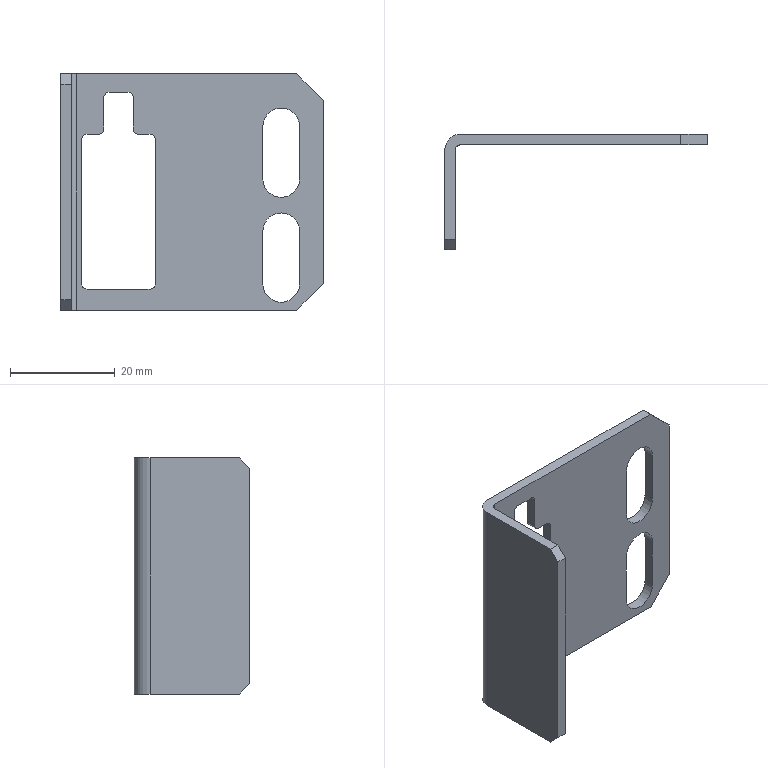Part | STEP file | 1358-7.stp.STEP | 1 solid | 40 faces | box 50 x 22 x 45 mm | volume 4817 mm3 | plane 24 | cylinder 16 | commonest cylinder face diameters 2 x9 7 x6 6 x1
STEP:
#1=CARTESIAN_POINT('',(0.,22.,20.));
#2=VERTEX_POINT('',#1);
#3=CARTESIAN_POINT('',(0.,5.,20.));
#4=VERTEX_POINT('',#3);
#5=CARTESIAN_POINT('',(0.,22.,20.));
#6=DIRECTION('',(0.,-1.,0.));
#7=VECTOR('',#6,1000.);
#8=LINE('',#5,#7);
#9=EDGE_CURVE('',#2,#4,#8,.T.);
#10=ORIENTED_EDGE('',*,*,#9,.T.);
#11=CARTESIAN_POINT('',(2.,5.,20.));
#12=VERTEX_POINT('',#11);
#13=CARTESIAN_POINT('',(2.,5.,20.));
#14=DIRECTION('',(-1.,0.,0.));
#15=VECTOR('',#14,1000.);
#16=LINE('',#13,#15);
#17=EDGE_CURVE('',#12,#4,#16,.T.);
#18=ORIENTED_EDGE('',*,*,#17,.F.);
#19=CARTESIAN_POINT('',(2.,22.,20.));
#20=VERTEX_POINT('',#19);
#21=CARTESIAN_POINT('',(2.,22.,20.));
#22=DIRECTION('',(0.,-1.,0.));
#23=VECTOR('',#22,1000.);
#24=LINE('',#21,#23);
#25=EDGE_CURVE('',#20,#12,#24,.T.);
#26=ORIENTED_EDGE('',*,*,#25,.F.);
#27=CARTESIAN_POINT('',(3.,23.,20.));
#28=VERTEX_POINT('',#27);
#29=CARTESIAN_POINT('',(3.,22.,20.));
#30=DIRECTION('',(0.,0.,-1.));
#31=DIRECTION('',(-1.,0.,0.));
#32=AXIS2_PLACEMENT_3D('',#29,#30,#31);
#33=CIRCLE('',#32,1.);
#34=EDGE_CURVE('',#20,#28,#33,.T.);
#35=ORIENTED_EDGE('',*,*,#34,.T.);
#36=CARTESIAN_POINT('',(45.,23.,20.));
#37=VERTEX_POINT('',#36);
#38=CARTESIAN_POINT('',(3.,23.,20.));
#39=DIRECTION('',(1.,0.,0.));
#40=VECTOR('',#39,1000.);
#41=LINE('',#38,#40);
#42=EDGE_CURVE('',#28,#37,#41,.T.);
#43=ORIENTED_EDGE('',*,*,#42,.T.);
#44=CARTESIAN_POINT('',(45.,25.,20.));
#45=VERTEX_POINT('',#44);
#46=CARTESIAN_POINT('',(45.,25.,20.));
#47=DIRECTION('',(0.,-1.,0.));
#48=VECTOR('',#47,1000.);
#49=LINE('',#46,#48);
#50=EDGE_CURVE('',#45,#37,#49,.T.);
#51=ORIENTED_EDGE('',*,*,#50,.F.);
#52=CARTESIAN_POINT('',(3.,25.,20.));
#53=VERTEX_POINT('',#52);
#54=CARTESIAN_POINT('',(3.,25.,20.));
#55=DIRECTION('',(1.,0.,0.));
#56=VECTOR('',#55,1000.);
#57=LINE('',#54,#56);
#58=EDGE_CURVE('',#53,#45,#57,.T.);
#59=ORIENTED_EDGE('',*,*,#58,.F.);
#60=CARTESIAN_POINT('',(3.,22.,20.));
#61=DIRECTION('',(0.,0.,1.));
#62=DIRECTION('',(0.,1.,0.));
#63=AXIS2_PLACEMENT_3D('',#60,#61,#62);
#64=CIRCLE('',#63,3.);
#65=EDGE_CURVE('',#53,#2,#64,.T.);
#66=ORIENTED_EDGE('',*,*,#65,.T.);
#67=EDGE_LOOP('',(#10,#18,#26,#35,#43,#51,#59,#66));
#68=FACE_OUTER_BOUND('',#67,.T.);
#69=CARTESIAN_POINT('',(0.,0.,20.));
#70=DIRECTION('',(0.,0.,1.));
#71=DIRECTION('',(1.,0.,0.));
#72=AXIS2_PLACEMENT_3D('',#69,#70,#71);
#73=PLANE('',#72);
#74=ADVANCED_FACE('',(#68),#73,.T.);
#75=CARTESIAN_POINT('',(3.,25.,-25.));
#76=VERTEX_POINT('',#75);
#77=CARTESIAN_POINT('',(3.,25.,-25.));
#78=DIRECTION('',(0.,0.,1.));
#79=VECTOR('',#78,1000.);
#80=LINE('',#77,#79);
#81=EDGE_CURVE('',#76,#53,#80,.T.);
#82=ORIENTED_EDGE('',*,*,#81,.F.);
#83=CARTESIAN_POINT('',(0.,22.,-25.));
#84=VERTEX_POINT('',#83);
#85=CARTESIAN_POINT('',(3.,22.,-25.));
#86=DIRECTION('',(0.,0.,-1.));
#87=DIRECTION('',(-1.,0.,0.));
#88=AXIS2_PLACEMENT_3D('',#85,#86,#87);
#89=CIRCLE('',#88,3.);
#90=EDGE_CURVE('',#84,#76,#89,.T.);
#91=ORIENTED_EDGE('',*,*,#90,.F.);
#92=CARTESIAN_POINT('',(0.,22.,-25.));
#93=DIRECTION('',(0.,0.,1.));
#94=VECTOR('',#93,1000.);
#95=LINE('',#92,#94);
#96=EDGE_CURVE('',#84,#2,#95,.T.);
#97=ORIENTED_EDGE('',*,*,#96,.T.);
#98=ORIENTED_EDGE('',*,*,#65,.F.);
#99=EDGE_LOOP('',(#82,#91,#97,#98));
#100=FACE_OUTER_BOUND('',#99,.T.);
#101=CARTESIAN_POINT('',(3.,22.,-83.662));
#102=DIRECTION('',(0.,0.,1.));
#103=DIRECTION('',(0.,1.,0.));
#104=AXIS2_PLACEMENT_3D('',#101,#102,#103);
#105=CYLINDRICAL_SURFACE('',#104,3.);
#106=ADVANCED_FACE('',(#100),#105,.T.);
#107=CARTESIAN_POINT('',(0.,5.,-25.));
#108=VERTEX_POINT('',#107);
#109=CARTESIAN_POINT('',(0.,5.,-25.));
#110=DIRECTION('',(0.,1.,0.));
#111=VECTOR('',#110,1000.);
#112=LINE('',#109,#111);
#113=EDGE_CURVE('',#108,#84,#112,.T.);
#114=ORIENTED_EDGE('',*,*,#113,.F.);
#115=CARTESIAN_POINT('',(0.,3.,-23.));
#116=VERTEX_POINT('',#115);
#117=CARTESIAN_POINT('',(0.,5.,-25.));
#118=DIRECTION('',(0.,-0.7071,0.7071));
#119=VECTOR('',#118,1000.);
#120=LINE('',#117,#119);
#121=EDGE_CURVE('',#108,#116,#120,.T.);
#122=ORIENTED_EDGE('',*,*,#121,.T.);
#123=CARTESIAN_POINT('',(0.,3.,18.));
#124=VERTEX_POINT('',#123);
#125=CARTESIAN_POINT('',(0.,3.,18.));
#126=DIRECTION('',(0.,0.,-1.));
#127=VECTOR('',#126,1000.);
#128=LINE('',#125,#127);
#129=EDGE_CURVE('',#124,#116,#128,.T.);
#130=ORIENTED_EDGE('',*,*,#129,.F.);
#131=CARTESIAN_POINT('',(0.,3.,18.));
#132=DIRECTION('',(0.,0.7071,0.7071));
#133=VECTOR('',#132,1000.);
#134=LINE('',#131,#133);
#135=EDGE_CURVE('',#124,#4,#134,.T.);
#136=ORIENTED_EDGE('',*,*,#135,.T.);
#137=ORIENTED_EDGE('',*,*,#9,.F.);
#138=ORIENTED_EDGE('',*,*,#96,.F.);
#139=EDGE_LOOP('',(#114,#122,#130,#136,#137,#138));
#140=FACE_OUTER_BOUND('',#139,.T.);
#141=CARTESIAN_POINT('',(0.,25.,-20.));
#142=DIRECTION('',(-1.,0.,0.));
#143=DIRECTION('',(0.,0.,1.));
#144=AXIS2_PLACEMENT_3D('',#141,#142,#143);
#145=PLANE('',#144);
#146=ADVANCED_FACE('',(#140),#145,.T.);
#147=CARTESIAN_POINT('',(2.,3.,18.));
#148=VERTEX_POINT('',#147);
#149=CARTESIAN_POINT('',(2.,3.,18.));
#150=DIRECTION('',(-1.,0.,0.));
#151=VECTOR('',#150,1000.);
#152=LINE('',#149,#151);
#153=EDGE_CURVE('',#148,#124,#152,.T.);
#154=ORIENTED_EDGE('',*,*,#153,.F.);
#155=CARTESIAN_POINT('',(2.,5.,20.));
#156=DIRECTION('',(0.,-0.7071,-0.7071));
#157=VECTOR('',#156,1000.);
#158=LINE('',#155,#157);
#159=EDGE_CURVE('',#12,#148,#158,.T.);
#160=ORIENTED_EDGE('',*,*,#159,.F.);
#161=ORIENTED_EDGE('',*,*,#17,.T.);
#162=ORIENTED_EDGE('',*,*,#135,.F.);
#163=EDGE_LOOP('',(#154,#160,#161,#162));
#164=FACE_OUTER_BOUND('',#163,.T.);
#165=CARTESIAN_POINT('',(1.,4.,19.));
#166=DIRECTION('',(0.,-0.7071,0.7071));
#167=DIRECTION('',(-1.,0.,0.));
#168=AXIS2_PLACEMENT_3D('',#165,#166,#167);
#169=PLANE('',#168);
#170=ADVANCED_FACE('',(#164),#169,.T.);
#171=ORIENTED_EDGE('',*,*,#25,.T.);
#172=ORIENTED_EDGE('',*,*,#159,.T.);
#173=CARTESIAN_POINT('',(2.,3.,-23.));
#174=VERTEX_POINT('',#173);
#175=CARTESIAN_POINT('',(2.,3.,-23.));
#176=DIRECTION('',(0.,0.,1.));
#177=VECTOR('',#176,1000.);
#178=LINE('',#175,#177);
#179=EDGE_CURVE('',#174,#148,#178,.T.);
#180=ORIENTED_EDGE('',*,*,#179,.F.);
#181=CARTESIAN_POINT('',(2.,5.,-25.));
#182=VERTEX_POINT('',#181);
#183=CARTESIAN_POINT('',(2.,3.,-23.));
#184=DIRECTION('',(0.,0.7071,-0.7071));
#185=VECTOR('',#184,1000.);
#186=LINE('',#183,#185);
#187=EDGE_CURVE('',#174,#182,#186,.T.);
#188=ORIENTED_EDGE('',*,*,#187,.T.);
#189=CARTESIAN_POINT('',(2.,22.,-25.));
#190=VERTEX_POINT('',#189);
#191=CARTESIAN_POINT('',(2.,22.,-25.));
#192=DIRECTION('',(0.,-1.,0.));
#193=VECTOR('',#192,1000.);
#194=LINE('',#191,#193);
#195=EDGE_CURVE('',#190,#182,#194,.T.);
#196=ORIENTED_EDGE('',*,*,#195,.F.);
#197=CARTESIAN_POINT('',(2.,22.,-25.));
#198=DIRECTION('',(0.,0.,1.));
#199=VECTOR('',#198,1000.);
#200=LINE('',#197,#199);
#201=EDGE_CURVE('',#190,#20,#200,.T.);
#202=ORIENTED_EDGE('',*,*,#201,.T.);
#203=EDGE_LOOP('',(#171,#172,#180,#188,#196,#202));
#204=FACE_OUTER_BOUND('',#203,.T.);
#205=CARTESIAN_POINT('',(2.,23.,-25.));
#206=DIRECTION('',(1.,0.,0.));
#207=DIRECTION('',(0.,1.,0.));
#208=AXIS2_PLACEMENT_3D('',#205,#206,#207);
#209=PLANE('',#208);
#210=ADVANCED_FACE('',(#204),#209,.T.);
#211=ORIENTED_EDGE('',*,*,#34,.F.);
#212=ORIENTED_EDGE('',*,*,#201,.F.);
#213=CARTESIAN_POINT('',(3.,23.,-25.));
#214=VERTEX_POINT('',#213);
#215=CARTESIAN_POINT('',(3.,22.,-25.));
#216=DIRECTION('',(0.,0.,1.));
#217=DIRECTION('',(0.,1.,0.));
#218=AXIS2_PLACEMENT_3D('',#215,#216,#217);
#219=CIRCLE('',#218,1.);
#220=EDGE_CURVE('',#214,#190,#219,.T.);
#221=ORIENTED_EDGE('',*,*,#220,.F.);
#222=CARTESIAN_POINT('',(3.,23.,-25.));
#223=DIRECTION('',(0.,0.,1.));
#224=VECTOR('',#223,1000.);
#225=LINE('',#222,#224);
#226=EDGE_CURVE('',#214,#28,#225,.T.);
#227=ORIENTED_EDGE('',*,*,#226,.T.);
#228=EDGE_LOOP('',(#211,#212,#221,#227));
#229=FACE_OUTER_BOUND('',#228,.T.);
#230=CARTESIAN_POINT('',(3.,22.,-83.662));
#231=DIRECTION('',(0.,0.,1.));
#232=DIRECTION('',(0.,1.,0.));
#233=AXIS2_PLACEMENT_3D('',#230,#231,#232);
#234=CYLINDRICAL_SURFACE('',#233,1.);
#235=ADVANCED_FACE('',(#229),#234,.F.);
#236=CARTESIAN_POINT('',(38.5,23.,10.));
#237=VERTEX_POINT('',#236);
#238=CARTESIAN_POINT('',(38.5,23.,0.));
#239=VERTEX_POINT('',#238);
#240=CARTESIAN_POINT('',(38.5,23.,10.));
#241=DIRECTION('',(0.,0.,-1.));
#242=VECTOR('',#241,1000.);
#243=LINE('',#240,#242);
#244=EDGE_CURVE('',#237,#239,#243,.T.);
#245=ORIENTED_EDGE('',*,*,#244,.F.);
#246=CARTESIAN_POINT('',(42.,23.,13.5));
#247=VERTEX_POINT('',#246);
#248=CARTESIAN_POINT('',(42.,23.,10.));
#249=DIRECTION('',(0.,-1.,0.));
#250=DIRECTION('',(1.,0.,0.));
#251=AXIS2_PLACEMENT_3D('',#248,#249,#250);
#252=CIRCLE('',#251,3.5);
#253=EDGE_CURVE('',#247,#237,#252,.T.);
#254=ORIENTED_EDGE('',*,*,#253,.F.);
#255=CARTESIAN_POINT('',(45.5,23.,10.));
#256=VERTEX_POINT('',#255);
#257=CARTESIAN_POINT('',(42.,23.,10.));
#258=DIRECTION('',(0.,-1.,0.));
#259=DIRECTION('',(1.,0.,0.));
#260=AXIS2_PLACEMENT_3D('',#257,#258,#259);
#261=CIRCLE('',#260,3.5);
#262=EDGE_CURVE('',#256,#247,#261,.T.);
#263=ORIENTED_EDGE('',*,*,#262,.F.);
#264=CARTESIAN_POINT('',(45.5,23.,0.));
#265=VERTEX_POINT('',#264);
#266=CARTESIAN_POINT('',(45.5,23.,0.));
#267=DIRECTION('',(0.,0.,1.));
#268=VECTOR('',#267,1000.);
#269=LINE('',#266,#268);
#270=EDGE_CURVE('',#265,#256,#269,.T.);
#271=ORIENTED_EDGE('',*,*,#270,.F.);
#272=CARTESIAN_POINT('',(42.,23.,0.));
#273=DIRECTION('',(0.,-1.,0.));
#274=DIRECTION('',(-1.,0.,0.));
#275=AXIS2_PLACEMENT_3D('',#272,#273,#274);
#276=CIRCLE('',#275,3.5);
#277=EDGE_CURVE('',#239,#265,#276,.T.);
#278=ORIENTED_EDGE('',*,*,#277,.F.);
#279=EDGE_LOOP('',(#245,#254,#263,#271,#278));
#280=FACE_BOUND('',#279,.T.);
#281=CARTESIAN_POINT('',(38.5,23.,-10.));
#282=VERTEX_POINT('',#281);
#283=CARTESIAN_POINT('',(38.5,23.,-20.));
#284=VERTEX_POINT('',#283);
#285=CARTESIAN_POINT('',(38.5,23.,-10.));
#286=DIRECTION('',(0.,0.,-1.));
#287=VECTOR('',#286,1000.);
#288=LINE('',#285,#287);
#289=EDGE_CURVE('',#282,#284,#288,.T.);
#290=ORIENTED_EDGE('',*,*,#289,.F.);
#291=CARTESIAN_POINT('',(42.,23.,-6.5));
#292=VERTEX_POINT('',#291);
#293=CARTESIAN_POINT('',(42.,23.,-10.));
#294=DIRECTION('',(0.,-1.,0.));
#295=DIRECTION('',(1.,0.,0.));
#296=AXIS2_PLACEMENT_3D('',#293,#294,#295);
#297=CIRCLE('',#296,3.5);
#298=EDGE_CURVE('',#292,#282,#297,.T.);
#299=ORIENTED_EDGE('',*,*,#298,.F.);
#300=CARTESIAN_POINT('',(45.5,23.,-10.));
#301=VERTEX_POINT('',#300);
#302=CARTESIAN_POINT('',(42.,23.,-10.));
#303=DIRECTION('',(0.,-1.,0.));
#304=DIRECTION('',(1.,0.,0.));
#305=AXIS2_PLACEMENT_3D('',#302,#303,#304);
#306=CIRCLE('',#305,3.5);
#307=EDGE_CURVE('',#301,#292,#306,.T.);
#308=ORIENTED_EDGE('',*,*,#307,.F.);
#309=CARTESIAN_POINT('',(45.5,23.,-20.));
#310=VERTEX_POINT('',#309);
#311=CARTESIAN_POINT('',(45.5,23.,-20.));
#312=DIRECTION('',(0.,0.,1.));
#313=VECTOR('',#312,1000.);
#314=LINE('',#311,#313);
#315=EDGE_CURVE('',#310,#301,#314,.T.);
#316=ORIENTED_EDGE('',*,*,#315,.F.);
#317=CARTESIAN_POINT('',(42.,23.,-20.));
#318=DIRECTION('',(0.,-1.,0.));
#319=DIRECTION('',(-1.,0.,0.));
#320=AXIS2_PLACEMENT_3D('',#317,#318,#319);
#321=CIRCLE('',#320,3.5);
#322=EDGE_CURVE('',#284,#310,#321,.T.);
#323=ORIENTED_EDGE('',*,*,#322,.F.);
#324=EDGE_LOOP('',(#290,#299,#308,#316,#323));
#325=FACE_BOUND('',#324,.T.);
#326=CARTESIAN_POINT('',(17.,23.,8.5));
#327=VERTEX_POINT('',#326);
#328=CARTESIAN_POINT('',(14.8,23.,8.5));
#329=VERTEX_POINT('',#328);
#330=CARTESIAN_POINT('',(17.,23.,8.5));
#331=DIRECTION('',(-1.,0.,0.));
#332=VECTOR('',#331,1000.);
#333=LINE('',#330,#332);
#334=EDGE_CURVE('',#327,#329,#333,.T.);
#335=ORIENTED_EDGE('',*,*,#334,.F.);
#336=CARTESIAN_POINT('',(18.,23.,7.5));
#337=VERTEX_POINT('',#336);
#338=CARTESIAN_POINT('',(17.,23.,7.5));
#339=DIRECTION('',(0.,1.,0.));
#340=DIRECTION('',(0.,0.,1.));
#341=AXIS2_PLACEMENT_3D('',#338,#339,#340);
#342=CIRCLE('',#341,1.);
#343=EDGE_CURVE('',#327,#337,#342,.T.);
#344=ORIENTED_EDGE('',*,*,#343,.T.);
#345=CARTESIAN_POINT('',(18.,23.,-20.));
#346=VERTEX_POINT('',#345);
#347=CARTESIAN_POINT('',(18.,23.,-20.));
#348=DIRECTION('',(0.,0.,1.));
#349=VECTOR('',#348,1000.);
#350=LINE('',#347,#349);
#351=EDGE_CURVE('',#346,#337,#350,.T.);
#352=ORIENTED_EDGE('',*,*,#351,.F.);
#353=CARTESIAN_POINT('',(17.,23.,-21.));
#354=VERTEX_POINT('',#353);
#355=CARTESIAN_POINT('',(17.,23.,-20.));
#356=DIRECTION('',(0.,1.,0.));
#357=DIRECTION('',(1.,0.,0.));
#358=AXIS2_PLACEMENT_3D('',#355,#356,#357);
#359=CIRCLE('',#358,1.);
#360=EDGE_CURVE('',#346,#354,#359,.T.);
#361=ORIENTED_EDGE('',*,*,#360,.T.);
#362=CARTESIAN_POINT('',(5.,23.,-21.));
#363=VERTEX_POINT('',#362);
#364=CARTESIAN_POINT('',(5.,23.,-21.));
#365=DIRECTION('',(1.,0.,0.));
#366=VECTOR('',#365,1000.);
#367=LINE('',#364,#366);
#368=EDGE_CURVE('',#363,#354,#367,.T.);
#369=ORIENTED_EDGE('',*,*,#368,.F.);
#370=CARTESIAN_POINT('',(4.,23.,-20.));
#371=VERTEX_POINT('',#370);
#372=CARTESIAN_POINT('',(5.,23.,-20.));
#373=DIRECTION('',(0.,1.,0.));
#374=DIRECTION('',(0.,0.,-1.));
#375=AXIS2_PLACEMENT_3D('',#372,#373,#374);
#376=CIRCLE('',#375,1.);
#377=EDGE_CURVE('',#363,#371,#376,.T.);
#378=ORIENTED_EDGE('',*,*,#377,.T.);
#379=CARTESIAN_POINT('',(4.,23.,7.5));
#380=VERTEX_POINT('',#379);
#381=CARTESIAN_POINT('',(4.,23.,7.5));
#382=DIRECTION('',(0.,0.,-1.));
#383=VECTOR('',#382,1000.);
#384=LINE('',#381,#383);
#385=EDGE_CURVE('',#380,#371,#384,.T.);
#386=ORIENTED_EDGE('',*,*,#385,.F.);
#387=CARTESIAN_POINT('',(5.,23.,8.5));
#388=VERTEX_POINT('',#387);
#389=CARTESIAN_POINT('',(5.,23.,7.5));
#390=DIRECTION('',(0.,1.,0.));
#391=DIRECTION('',(-1.,0.,0.));
#392=AXIS2_PLACEMENT_3D('',#389,#390,#391);
#393=CIRCLE('',#392,1.);
#394=EDGE_CURVE('',#380,#388,#393,.T.);
#395=ORIENTED_EDGE('',*,*,#394,.T.);
#396=CARTESIAN_POINT('',(7.2,23.,8.5));
#397=VERTEX_POINT('',#396);
#398=CARTESIAN_POINT('',(7.2,23.,8.5));
#399=DIRECTION('',(-1.,0.,0.));
#400=VECTOR('',#399,1000.);
#401=LINE('',#398,#400);
#402=EDGE_CURVE('',#397,#388,#401,.T.);
#403=ORIENTED_EDGE('',*,*,#402,.F.);
#404=CARTESIAN_POINT('',(8.2,23.,9.5));
#405=VERTEX_POINT('',#404);
#406=CARTESIAN_POINT('',(7.2,23.,9.5));
#407=DIRECTION('',(0.,-1.,0.));
#408=DIRECTION('',(0.,0.,-1.));
#409=AXIS2_PLACEMENT_3D('',#406,#407,#408);
#410=CIRCLE('',#409,1.);
#411=EDGE_CURVE('',#397,#405,#410,.T.);
#412=ORIENTED_EDGE('',*,*,#411,.T.);
#413=CARTESIAN_POINT('',(8.2,23.,15.5));
#414=VERTEX_POINT('',#413);
#415=CARTESIAN_POINT('',(8.2,23.,15.5));
#416=DIRECTION('',(0.,0.,-1.));
#417=VECTOR('',#416,1000.);
#418=LINE('',#415,#417);
#419=EDGE_CURVE('',#414,#405,#418,.T.);
#420=ORIENTED_EDGE('',*,*,#419,.F.);
#421=CARTESIAN_POINT('',(9.2,23.,16.5));
#422=VERTEX_POINT('',#421);
#423=CARTESIAN_POINT('',(9.2,23.,15.5));
#424=DIRECTION('',(0.,1.,0.));
#425=DIRECTION('',(-1.,0.,0.));
#426=AXIS2_PLACEMENT_3D('',#423,#424,#425);
#427=CIRCLE('',#426,1.);
#428=EDGE_CURVE('',#414,#422,#427,.T.);
#429=ORIENTED_EDGE('',*,*,#428,.T.);
#430=CARTESIAN_POINT('',(12.8,23.,16.5));
#431=VERTEX_POINT('',#430);
#432=CARTESIAN_POINT('',(12.8,23.,16.5));
#433=DIRECTION('',(-1.,0.,0.));
#434=VECTOR('',#433,1000.);
#435=LINE('',#432,#434);
#436=EDGE_CURVE('',#431,#422,#435,.T.);
#437=ORIENTED_EDGE('',*,*,#436,.F.);
#438=CARTESIAN_POINT('',(13.8,23.,15.5));
#439=VERTEX_POINT('',#438);
#440=CARTESIAN_POINT('',(12.8,23.,15.5));
#441=DIRECTION('',(0.,1.,0.));
#442=DIRECTION('',(0.,0.,1.));
#443=AXIS2_PLACEMENT_3D('',#440,#441,#442);
#444=CIRCLE('',#443,1.);
#445=EDGE_CURVE('',#431,#439,#444,.T.);
#446=ORIENTED_EDGE('',*,*,#445,.T.);
#447=CARTESIAN_POINT('',(13.8,23.,9.5));
#448=VERTEX_POINT('',#447);
#449=CARTESIAN_POINT('',(13.8,23.,9.5));
#450=DIRECTION('',(0.,0.,1.));
#451=VECTOR('',#450,1000.);
#452=LINE('',#449,#451);
#453=EDGE_CURVE('',#448,#439,#452,.T.);
#454=ORIENTED_EDGE('',*,*,#453,.F.);
#455=CARTESIAN_POINT('',(14.8,23.,9.5));
#456=DIRECTION('',(0.,-1.,0.));
#457=DIRECTION('',(-1.,0.,0.));
#458=AXIS2_PLACEMENT_3D('',#455,#456,#457);
#459=CIRCLE('',#458,1.);
#460=EDGE_CURVE('',#448,#329,#459,.T.);
#461=ORIENTED_EDGE('',*,*,#460,.T.);
#462=EDGE_LOOP('',(#335,#344,#352,#361,#369,#378,#386,#395,#403,#412,#420,#429,#437,#446,#454,#461));
#463=FACE_BOUND('',#462,.T.);
#464=CARTESIAN_POINT('',(45.,23.,-25.));
#465=VERTEX_POINT('',#464);
#466=CARTESIAN_POINT('',(45.,23.,-25.));
#467=DIRECTION('',(-1.,0.,0.));
#468=VECTOR('',#467,1000.);
#469=LINE('',#466,#468);
#470=EDGE_CURVE('',#465,#214,#469,.T.);
#471=ORIENTED_EDGE('',*,*,#470,.F.);
#472=CARTESIAN_POINT('',(50.,23.,-20.));
#473=VERTEX_POINT('',#472);
#474=CARTESIAN_POINT('',(45.,23.,-25.));
#475=DIRECTION('',(0.7071,0.,0.7071));
#476=VECTOR('',#475,1000.);
#477=LINE('',#474,#476);
#478=EDGE_CURVE('',#465,#473,#477,.T.);
#479=ORIENTED_EDGE('',*,*,#478,.T.);
#480=CARTESIAN_POINT('',(50.,23.,15.));
#481=VERTEX_POINT('',#480);
#482=CARTESIAN_POINT('',(50.,23.,15.));
#483=DIRECTION('',(0.,0.,-1.));
#484=VECTOR('',#483,1000.);
#485=LINE('',#482,#484);
#486=EDGE_CURVE('',#481,#473,#485,.T.);
#487=ORIENTED_EDGE('',*,*,#486,.F.);
#488=CARTESIAN_POINT('',(50.,23.,15.));
#489=DIRECTION('',(-0.7071,0.,0.7071));
#490=VECTOR('',#489,1000.);
#491=LINE('',#488,#490);
#492=EDGE_CURVE('',#481,#37,#491,.T.);
#493=ORIENTED_EDGE('',*,*,#492,.T.);
#494=ORIENTED_EDGE('',*,*,#42,.F.);
#495=ORIENTED_EDGE('',*,*,#226,.F.);
#496=EDGE_LOOP('',(#471,#479,#487,#493,#494,#495));
#497=FACE_OUTER_BOUND('',#496,.T.);
#498=CARTESIAN_POINT('',(0.,23.,-20.));
#499=DIRECTION('',(0.,-1.,0.));
#500=DIRECTION('',(0.,0.,-1.));
#501=AXIS2_PLACEMENT_3D('',#498,#499,#500);
#502=PLANE('',#501);
#503=ADVANCED_FACE('',(#280,#325,#463,#497),#502,.T.);
#504=CARTESIAN_POINT('',(13.8,25.,9.5));
#505=VERTEX_POINT('',#504);
#506=CARTESIAN_POINT('',(13.8,25.,9.5));
#507=DIRECTION('',(0.,-1.,0.));
#508=VECTOR('',#507,1000.);
#509=LINE('',#506,#508);
#510=EDGE_CURVE('',#505,#448,#509,.T.);
#511=ORIENTED_EDGE('',*,*,#510,.F.);
#512=CARTESIAN_POINT('',(14.8,25.,8.5));
#513=VERTEX_POINT('',#512);
#514=CARTESIAN_POINT('',(14.8,25.,9.5));
#515=DIRECTION('',(0.,1.,0.));
#516=DIRECTION('',(0.,0.,-1.));
#517=AXIS2_PLACEMENT_3D('',#514,#515,#516);
#518=CIRCLE('',#517,1.);
#519=EDGE_CURVE('',#513,#505,#518,.T.);
#520=ORIENTED_EDGE('',*,*,#519,.F.);
#521=CARTESIAN_POINT('',(14.8,25.,8.5));
#522=DIRECTION('',(0.,-1.,0.));
#523=VECTOR('',#522,1000.);
#524=LINE('',#521,#523);
#525=EDGE_CURVE('',#513,#329,#524,.T.);
#526=ORIENTED_EDGE('',*,*,#525,.T.);
#527=ORIENTED_EDGE('',*,*,#460,.F.);
#528=EDGE_LOOP('',(#511,#520,#526,#527));
#529=FACE_OUTER_BOUND('',#528,.T.);
#530=CARTESIAN_POINT('',(14.8,27.607,9.5));
#531=DIRECTION('',(0.,-1.,0.));
#532=DIRECTION('',(-1.,0.,0.));
#533=AXIS2_PLACEMENT_3D('',#530,#531,#532);
#534=CYLINDRICAL_SURFACE('',#533,1.);
#535=ADVANCED_FACE('',(#529),#534,.T.);
#536=CARTESIAN_POINT('',(17.,25.,8.5));
#537=VERTEX_POINT('',#536);
#538=CARTESIAN_POINT('',(17.,25.,8.5));
#539=DIRECTION('',(-1.,0.,0.));
#540=VECTOR('',#539,1000.);
#541=LINE('',#538,#540);
#542=EDGE_CURVE('',#537,#513,#541,.T.);
#543=ORIENTED_EDGE('',*,*,#542,.F.);
#544=CARTESIAN_POINT('',(17.,23.,8.5));
#545=DIRECTION('',(0.,1.,0.));
#546=VECTOR('',#545,1000.);
#547=LINE('',#544,#546);
#548=EDGE_CURVE('',#327,#537,#547,.T.);
#549=ORIENTED_EDGE('',*,*,#548,.F.);
#550=ORIENTED_EDGE('',*,*,#334,.T.);
#551=ORIENTED_EDGE('',*,*,#525,.F.);
#552=EDGE_LOOP('',(#543,#549,#550,#551));
#553=FACE_OUTER_BOUND('',#552,.T.);
#554=CARTESIAN_POINT('',(18.,23.,8.5));
#555=DIRECTION('',(0.,0.,1.));
#556=DIRECTION('',(1.,0.,0.));
#557=AXIS2_PLACEMENT_3D('',#554,#555,#556);
#558=PLANE('',#557);
#559=ADVANCED_FACE('',(#553),#558,.F.);
#560=CARTESIAN_POINT('',(18.,25.,7.5));
#561=VERTEX_POINT('',#560);
#562=CARTESIAN_POINT('',(17.,25.,7.5));
#563=DIRECTION('',(0.,-1.,0.));
#564=DIRECTION('',(1.,0.,0.));
#565=AXIS2_PLACEMENT_3D('',#562,#563,#564);
#566=CIRCLE('',#565,1.);
#567=EDGE_CURVE('',#561,#537,#566,.T.);
#568=ORIENTED_EDGE('',*,*,#567,.F.);
#569=CARTESIAN_POINT('',(18.,23.,7.5));
#570=DIRECTION('',(0.,1.,0.));
#571=VECTOR('',#570,1000.);
#572=LINE('',#569,#571);
#573=EDGE_CURVE('',#337,#561,#572,.T.);
#574=ORIENTED_EDGE('',*,*,#573,.F.);
#575=ORIENTED_EDGE('',*,*,#343,.F.);
#576=ORIENTED_EDGE('',*,*,#548,.T.);
#577=EDGE_LOOP('',(#568,#574,#575,#576));
#578=FACE_OUTER_BOUND('',#577,.T.);
#579=CARTESIAN_POINT('',(17.,20.393,7.5));
#580=DIRECTION('',(0.,1.,0.));
#581=DIRECTION('',(0.,0.,1.));
#582=AXIS2_PLACEMENT_3D('',#579,#580,#581);
#583=CYLINDRICAL_SURFACE('',#582,1.);
#584=ADVANCED_FACE('',(#578),#583,.F.);
#585=CARTESIAN_POINT('',(18.,25.,-20.));
#586=VERTEX_POINT('',#585);
#587=CARTESIAN_POINT('',(18.,25.,-20.));
#588=DIRECTION('',(0.,0.,1.));
#589=VECTOR('',#588,1000.);
#590=LINE('',#587,#589);
#591=EDGE_CURVE('',#586,#561,#590,.T.);
#592=ORIENTED_EDGE('',*,*,#591,.F.);
#593=CARTESIAN_POINT('',(18.,23.,-20.));
#594=DIRECTION('',(0.,1.,0.));
#595=VECTOR('',#594,1000.);
#596=LINE('',#593,#595);
#597=EDGE_CURVE('',#346,#586,#596,.T.);
#598=ORIENTED_EDGE('',*,*,#597,.F.);
#599=ORIENTED_EDGE('',*,*,#351,.T.);
#600=ORIENTED_EDGE('',*,*,#573,.T.);
#601=EDGE_LOOP('',(#592,#598,#599,#600));
#602=FACE_OUTER_BOUND('',#601,.T.);
#603=CARTESIAN_POINT('',(18.,23.,-21.));
#604=DIRECTION('',(1.,0.,0.));
#605=DIRECTION('',(0.,1.,0.));
#606=AXIS2_PLACEMENT_3D('',#603,#604,#605);
#607=PLANE('',#606);
#608=ADVANCED_FACE('',(#602),#607,.F.);
#609=ORIENTED_EDGE('',*,*,#597,.T.);
#610=CARTESIAN_POINT('',(17.,25.,-21.));
#611=VERTEX_POINT('',#610);
#612=CARTESIAN_POINT('',(17.,25.,-20.));
#613=DIRECTION('',(0.,-1.,0.));
#614=DIRECTION('',(0.,0.,-1.));
#615=AXIS2_PLACEMENT_3D('',#612,#613,#614);
#616=CIRCLE('',#615,1.);
#617=EDGE_CURVE('',#611,#586,#616,.T.);
#618=ORIENTED_EDGE('',*,*,#617,.F.);
#619=CARTESIAN_POINT('',(17.,23.,-21.));
#620=DIRECTION('',(0.,1.,0.));
#621=VECTOR('',#620,1000.);
#622=LINE('',#619,#621);
#623=EDGE_CURVE('',#354,#611,#622,.T.);
#624=ORIENTED_EDGE('',*,*,#623,.F.);
#625=ORIENTED_EDGE('',*,*,#360,.F.);
#626=EDGE_LOOP('',(#609,#618,#624,#625));
#627=FACE_OUTER_BOUND('',#626,.T.);
#628=CARTESIAN_POINT('',(17.,20.393,-20.));
#629=DIRECTION('',(0.,1.,0.));
#630=DIRECTION('',(1.,0.,0.));
#631=AXIS2_PLACEMENT_3D('',#628,#629,#630);
#632=CYLINDRICAL_SURFACE('',#631,1.);
#633=ADVANCED_FACE('',(#627),#632,.F.);
#634=ORIENTED_EDGE('',*,*,#368,.T.);
#635=ORIENTED_EDGE('',*,*,#623,.T.);
#636=CARTESIAN_POINT('',(5.,25.,-21.));
#637=VERTEX_POINT('',#636);
#638=CARTESIAN_POINT('',(5.,25.,-21.));
#639=DIRECTION('',(1.,0.,0.));
#640=VECTOR('',#639,1000.);
#641=LINE('',#638,#640);
#642=EDGE_CURVE('',#637,#611,#641,.T.);
#643=ORIENTED_EDGE('',*,*,#642,.F.);
#644=CARTESIAN_POINT('',(5.,23.,-21.));
#645=DIRECTION('',(0.,1.,0.));
#646=VECTOR('',#645,1000.);
#647=LINE('',#644,#646);
#648=EDGE_CURVE('',#363,#637,#647,.T.);
#649=ORIENTED_EDGE('',*,*,#648,.F.);
#650=EDGE_LOOP('',(#634,#635,#643,#649));
#651=FACE_OUTER_BOUND('',#650,.T.);
#652=CARTESIAN_POINT('',(4.,23.,-21.));
#653=DIRECTION('',(0.,0.,-1.));
#654=DIRECTION('',(0.,-1.,0.));
#655=AXIS2_PLACEMENT_3D('',#652,#653,#654);
#656=PLANE('',#655);
#657=ADVANCED_FACE('',(#651),#656,.F.);
#658=ORIENTED_EDGE('',*,*,#648,.T.);
#659=CARTESIAN_POINT('',(4.,25.,-20.));
#660=VERTEX_POINT('',#659);
#661=CARTESIAN_POINT('',(5.,25.,-20.));
#662=DIRECTION('',(0.,-1.,0.));
#663=DIRECTION('',(-1.,0.,0.));
#664=AXIS2_PLACEMENT_3D('',#661,#662,#663);
#665=CIRCLE('',#664,1.);
#666=EDGE_CURVE('',#660,#637,#665,.T.);
#667=ORIENTED_EDGE('',*,*,#666,.F.);
#668=CARTESIAN_POINT('',(4.,23.,-20.));
#669=DIRECTION('',(0.,1.,0.));
#670=VECTOR('',#669,1000.);
#671=LINE('',#668,#670);
#672=EDGE_CURVE('',#371,#660,#671,.T.);
#673=ORIENTED_EDGE('',*,*,#672,.F.);
#674=ORIENTED_EDGE('',*,*,#377,.F.);
#675=EDGE_LOOP('',(#658,#667,#673,#674));
#676=FACE_OUTER_BOUND('',#675,.T.);
#677=CARTESIAN_POINT('',(5.,20.393,-20.));
#678=DIRECTION('',(0.,1.,0.));
#679=DIRECTION('',(0.,0.,-1.));
#680=AXIS2_PLACEMENT_3D('',#677,#678,#679);
#681=CYLINDRICAL_SURFACE('',#680,1.);
#682=ADVANCED_FACE('',(#676),#681,.F.);
#683=ORIENTED_EDGE('',*,*,#385,.T.);
#684=ORIENTED_EDGE('',*,*,#672,.T.);
#685=CARTESIAN_POINT('',(4.,25.,7.5));
#686=VERTEX_POINT('',#685);
#687=CARTESIAN_POINT('',(4.,25.,7.5));
#688=DIRECTION('',(0.,0.,-1.));
#689=VECTOR('',#688,1000.);
#690=LINE('',#687,#689);
#691=EDGE_CURVE('',#686,#660,#690,.T.);
#692=ORIENTED_EDGE('',*,*,#691,.F.);
#693=CARTESIAN_POINT('',(4.,23.,7.5));
#694=DIRECTION('',(0.,1.,0.));
#695=VECTOR('',#694,1000.);
#696=LINE('',#693,#695);
#697=EDGE_CURVE('',#380,#686,#696,.T.);
#698=ORIENTED_EDGE('',*,*,#697,.F.);
#699=EDGE_LOOP('',(#683,#684,#692,#698));
#700=FACE_OUTER_BOUND('',#699,.T.);
#701=CARTESIAN_POINT('',(4.,23.,8.5));
#702=DIRECTION('',(-1.,0.,0.));
#703=DIRECTION('',(0.,0.,1.));
#704=AXIS2_PLACEMENT_3D('',#701,#702,#703);
#705=PLANE('',#704);
#706=ADVANCED_FACE('',(#700),#705,.F.);
#707=CARTESIAN_POINT('',(5.,25.,8.5));
#708=VERTEX_POINT('',#707);
#709=CARTESIAN_POINT('',(5.,25.,7.5));
#710=DIRECTION('',(0.,-1.,0.));
#711=DIRECTION('',(0.,0.,1.));
#712=AXIS2_PLACEMENT_3D('',#709,#710,#711);
#713=CIRCLE('',#712,1.);
#714=EDGE_CURVE('',#708,#686,#713,.T.);
#715=ORIENTED_EDGE('',*,*,#714,.F.);
#716=CARTESIAN_POINT('',(5.,23.,8.5));
#717=DIRECTION('',(0.,1.,0.));
#718=VECTOR('',#717,1000.);
#719=LINE('',#716,#718);
#720=EDGE_CURVE('',#388,#708,#719,.T.);
#721=ORIENTED_EDGE('',*,*,#720,.F.);
#722=ORIENTED_EDGE('',*,*,#394,.F.);
#723=ORIENTED_EDGE('',*,*,#697,.T.);
#724=EDGE_LOOP('',(#715,#721,#722,#723));
#725=FACE_OUTER_BOUND('',#724,.T.);
#726=CARTESIAN_POINT('',(5.,20.393,7.5));
#727=DIRECTION('',(0.,1.,0.));
#728=DIRECTION('',(-1.,0.,0.));
#729=AXIS2_PLACEMENT_3D('',#726,#727,#728);
#730=CYLINDRICAL_SURFACE('',#729,1.);
#731=ADVANCED_FACE('',(#725),#730,.F.);
#732=ORIENTED_EDGE('',*,*,#402,.T.);
#733=ORIENTED_EDGE('',*,*,#720,.T.);
#734=CARTESIAN_POINT('',(7.2,25.,8.5));
#735=VERTEX_POINT('',#734);
#736=CARTESIAN_POINT('',(7.2,25.,8.5));
#737=DIRECTION('',(-1.,0.,0.));
#738=VECTOR('',#737,1000.);
#739=LINE('',#736,#738);
#740=EDGE_CURVE('',#735,#708,#739,.T.);
#741=ORIENTED_EDGE('',*,*,#740,.F.);
#742=CARTESIAN_POINT('',(7.2,25.,8.5));
#743=DIRECTION('',(0.,-1.,0.));
#744=VECTOR('',#743,1000.);
#745=LINE('',#742,#744);
#746=EDGE_CURVE('',#735,#397,#745,.T.);
#747=ORIENTED_EDGE('',*,*,#746,.T.);
#748=EDGE_LOOP('',(#732,#733,#741,#747));
#749=FACE_OUTER_BOUND('',#748,.T.);
#750=CARTESIAN_POINT('',(8.2,23.,8.5));
#751=DIRECTION('',(0.,0.,1.));
#752=DIRECTION('',(1.,0.,0.));
#753=AXIS2_PLACEMENT_3D('',#750,#751,#752);
#754=PLANE('',#753);
#755=ADVANCED_FACE('',(#749),#754,.F.);
#756=ORIENTED_EDGE('',*,*,#746,.F.);
#757=CARTESIAN_POINT('',(8.2,25.,9.5));
#758=VERTEX_POINT('',#757);
#759=CARTESIAN_POINT('',(7.2,25.,9.5));
#760=DIRECTION('',(0.,1.,0.));
#761=DIRECTION('',(1.,0.,0.));
#762=AXIS2_PLACEMENT_3D('',#759,#760,#761);
#763=CIRCLE('',#762,1.);
#764=EDGE_CURVE('',#758,#735,#763,.T.);
#765=ORIENTED_EDGE('',*,*,#764,.F.);
#766=CARTESIAN_POINT('',(8.2,25.,9.5));
#767=DIRECTION('',(0.,-1.,0.));
#768=VECTOR('',#767,1000.);
#769=LINE('',#766,#768);
#770=EDGE_CURVE('',#758,#405,#769,.T.);
#771=ORIENTED_EDGE('',*,*,#770,.T.);
#772=ORIENTED_EDGE('',*,*,#411,.F.);
#773=EDGE_LOOP('',(#756,#765,#771,#772));
#774=FACE_OUTER_BOUND('',#773,.T.);
#775=CARTESIAN_POINT('',(7.2,27.607,9.5));
#776=DIRECTION('',(0.,-1.,0.));
#777=DIRECTION('',(0.,0.,-1.));
#778=AXIS2_PLACEMENT_3D('',#775,#776,#777);
#779=CYLINDRICAL_SURFACE('',#778,1.);
#780=ADVANCED_FACE('',(#774),#779,.T.);
#781=CARTESIAN_POINT('',(8.2,25.,15.5));
#782=VERTEX_POINT('',#781);
#783=CARTESIAN_POINT('',(8.2,25.,15.5));
#784=DIRECTION('',(0.,0.,-1.));
#785=VECTOR('',#784,1000.);
#786=LINE('',#783,#785);
#787=EDGE_CURVE('',#782,#758,#786,.T.);
#788=ORIENTED_EDGE('',*,*,#787,.F.);
#789=CARTESIAN_POINT('',(8.2,23.,15.5));
#790=DIRECTION('',(0.,1.,0.));
#791=VECTOR('',#790,1000.);
#792=LINE('',#789,#791);
#793=EDGE_CURVE('',#414,#782,#792,.T.);
#794=ORIENTED_EDGE('',*,*,#793,.F.);
#795=ORIENTED_EDGE('',*,*,#419,.T.);
#796=ORIENTED_EDGE('',*,*,#770,.F.);
#797=EDGE_LOOP('',(#788,#794,#795,#796));
#798=FACE_OUTER_BOUND('',#797,.T.);
#799=CARTESIAN_POINT('',(8.2,23.,16.5));
#800=DIRECTION('',(-1.,0.,0.));
#801=DIRECTION('',(0.,0.,1.));
#802=AXIS2_PLACEMENT_3D('',#799,#800,#801);
#803=PLANE('',#802);
#804=ADVANCED_FACE('',(#798),#803,.F.);
#805=CARTESIAN_POINT('',(9.2,25.,16.5));
#806=VERTEX_POINT('',#805);
#807=CARTESIAN_POINT('',(9.2,25.,15.5));
#808=DIRECTION('',(0.,-1.,0.));
#809=DIRECTION('',(0.,0.,1.));
#810=AXIS2_PLACEMENT_3D('',#807,#808,#809);
#811=CIRCLE('',#810,1.);
#812=EDGE_CURVE('',#806,#782,#811,.T.);
#813=ORIENTED_EDGE('',*,*,#812,.F.);
#814=CARTESIAN_POINT('',(9.2,23.,16.5));
#815=DIRECTION('',(0.,1.,0.));
#816=VECTOR('',#815,1000.);
#817=LINE('',#814,#816);
#818=EDGE_CURVE('',#422,#806,#817,.T.);
#819=ORIENTED_EDGE('',*,*,#818,.F.);
#820=ORIENTED_EDGE('',*,*,#428,.F.);
#821=ORIENTED_EDGE('',*,*,#793,.T.);
#822=EDGE_LOOP('',(#813,#819,#820,#821));
#823=FACE_OUTER_BOUND('',#822,.T.);
#824=CARTESIAN_POINT('',(9.2,20.393,15.5));
#825=DIRECTION('',(0.,1.,0.));
#826=DIRECTION('',(-1.,0.,0.));
#827=AXIS2_PLACEMENT_3D('',#824,#825,#826);
#828=CYLINDRICAL_SURFACE('',#827,1.);
#829=ADVANCED_FACE('',(#823),#828,.F.);
#830=CARTESIAN_POINT('',(12.8,25.,16.5));
#831=VERTEX_POINT('',#830);
#832=CARTESIAN_POINT('',(12.8,25.,16.5));
#833=DIRECTION('',(-1.,0.,0.));
#834=VECTOR('',#833,1000.);
#835=LINE('',#832,#834);
#836=EDGE_CURVE('',#831,#806,#835,.T.);
#837=ORIENTED_EDGE('',*,*,#836,.F.);
#838=CARTESIAN_POINT('',(12.8,23.,16.5));
#839=DIRECTION('',(0.,1.,0.));
#840=VECTOR('',#839,1000.);
#841=LINE('',#838,#840);
#842=EDGE_CURVE('',#431,#831,#841,.T.);
#843=ORIENTED_EDGE('',*,*,#842,.F.);
#844=ORIENTED_EDGE('',*,*,#436,.T.);
#845=ORIENTED_EDGE('',*,*,#818,.T.);
#846=EDGE_LOOP('',(#837,#843,#844,#845));
#847=FACE_OUTER_BOUND('',#846,.T.);
#848=CARTESIAN_POINT('',(13.8,23.,16.5));
#849=DIRECTION('',(0.,0.,1.));
#850=DIRECTION('',(1.,0.,0.));
#851=AXIS2_PLACEMENT_3D('',#848,#849,#850);
#852=PLANE('',#851);
#853=ADVANCED_FACE('',(#847),#852,.F.);
#854=CARTESIAN_POINT('',(13.8,25.,15.5));
#855=VERTEX_POINT('',#854);
#856=CARTESIAN_POINT('',(12.8,25.,15.5));
#857=DIRECTION('',(0.,-1.,0.));
#858=DIRECTION('',(1.,0.,0.));
#859=AXIS2_PLACEMENT_3D('',#856,#857,#858);
#860=CIRCLE('',#859,1.);
#861=EDGE_CURVE('',#855,#831,#860,.T.);
#862=ORIENTED_EDGE('',*,*,#861,.F.);
#863=CARTESIAN_POINT('',(13.8,23.,15.5));
#864=DIRECTION('',(0.,1.,0.));
#865=VECTOR('',#864,1000.);
#866=LINE('',#863,#865);
#867=EDGE_CURVE('',#439,#855,#866,.T.);
#868=ORIENTED_EDGE('',*,*,#867,.F.);
#869=ORIENTED_EDGE('',*,*,#445,.F.);
#870=ORIENTED_EDGE('',*,*,#842,.T.);
#871=EDGE_LOOP('',(#862,#868,#869,#870));
#872=FACE_OUTER_BOUND('',#871,.T.);
#873=CARTESIAN_POINT('',(12.8,20.393,15.5));
#874=DIRECTION('',(0.,1.,0.));
#875=DIRECTION('',(0.,0.,1.));
#876=AXIS2_PLACEMENT_3D('',#873,#874,#875);
#877=CYLINDRICAL_SURFACE('',#876,1.);
#878=ADVANCED_FACE('',(#872),#877,.F.);
#879=ORIENTED_EDGE('',*,*,#453,.T.);
#880=ORIENTED_EDGE('',*,*,#867,.T.);
#881=CARTESIAN_POINT('',(13.8,25.,9.5));
#882=DIRECTION('',(0.,0.,1.));
#883=VECTOR('',#882,1000.);
#884=LINE('',#881,#883);
#885=EDGE_CURVE('',#505,#855,#884,.T.);
#886=ORIENTED_EDGE('',*,*,#885,.F.);
#887=ORIENTED_EDGE('',*,*,#510,.T.);
#888=EDGE_LOOP('',(#879,#880,#886,#887));
#889=FACE_OUTER_BOUND('',#888,.T.);
#890=CARTESIAN_POINT('',(13.8,23.,8.5));
#891=DIRECTION('',(1.,0.,0.));
#892=DIRECTION('',(0.,1.,0.));
#893=AXIS2_PLACEMENT_3D('',#890,#891,#892);
#894=PLANE('',#893);
#895=ADVANCED_FACE('',(#889),#894,.F.);
#896=CARTESIAN_POINT('',(45.5,25.,0.));
#897=VERTEX_POINT('',#896);
#898=CARTESIAN_POINT('',(45.5,25.,10.));
#899=VERTEX_POINT('',#898);
#900=CARTESIAN_POINT('',(45.5,25.,0.));
#901=DIRECTION('',(0.,0.,1.));
#902=VECTOR('',#901,1000.);
#903=LINE('',#900,#902);
#904=EDGE_CURVE('',#897,#899,#903,.T.);
#905=ORIENTED_EDGE('',*,*,#904,.T.);
#906=CARTESIAN_POINT('',(42.,25.,13.5));
#907=VERTEX_POINT('',#906);
#908=CARTESIAN_POINT('',(42.,25.,10.));
#909=DIRECTION('',(0.,-1.,0.));
#910=DIRECTION('',(1.,0.,0.));
#911=AXIS2_PLACEMENT_3D('',#908,#909,#910);
#912=CIRCLE('',#911,3.5);
#913=EDGE_CURVE('',#899,#907,#912,.T.);
#914=ORIENTED_EDGE('',*,*,#913,.T.);
#915=CARTESIAN_POINT('',(38.5,25.,10.));
#916=VERTEX_POINT('',#915);
#917=CARTESIAN_POINT('',(42.,25.,10.));
#918=DIRECTION('',(0.,-1.,0.));
#919=DIRECTION('',(1.,0.,0.));
#920=AXIS2_PLACEMENT_3D('',#917,#918,#919);
#921=CIRCLE('',#920,3.5);
#922=EDGE_CURVE('',#907,#916,#921,.T.);
#923=ORIENTED_EDGE('',*,*,#922,.T.);
#924=CARTESIAN_POINT('',(38.5,25.,0.));
#925=VERTEX_POINT('',#924);
#926=CARTESIAN_POINT('',(38.5,25.,10.));
#927=DIRECTION('',(0.,0.,-1.));
#928=VECTOR('',#927,1000.);
#929=LINE('',#926,#928);
#930=EDGE_CURVE('',#916,#925,#929,.T.);
#931=ORIENTED_EDGE('',*,*,#930,.T.);
#932=CARTESIAN_POINT('',(42.,25.,0.));
#933=DIRECTION('',(0.,-1.,0.));
#934=DIRECTION('',(-1.,0.,0.));
#935=AXIS2_PLACEMENT_3D('',#932,#933,#934);
#936=CIRCLE('',#935,3.5);
#937=EDGE_CURVE('',#925,#897,#936,.T.);
#938=ORIENTED_EDGE('',*,*,#937,.T.);
#939=EDGE_LOOP('',(#905,#914,#923,#931,#938));
#940=FACE_BOUND('',#939,.T.);
#941=CARTESIAN_POINT('',(45.5,25.,-20.));
#942=VERTEX_POINT('',#941);
#943=CARTESIAN_POINT('',(45.5,25.,-10.));
#944=VERTEX_POINT('',#943);
#945=CARTESIAN_POINT('',(45.5,25.,-20.));
#946=DIRECTION('',(0.,0.,1.));
#947=VECTOR('',#946,1000.);
#948=LINE('',#945,#947);
#949=EDGE_CURVE('',#942,#944,#948,.T.);
#950=ORIENTED_EDGE('',*,*,#949,.T.);
#951=CARTESIAN_POINT('',(42.,25.,-6.5));
#952=VERTEX_POINT('',#951);
#953=CARTESIAN_POINT('',(42.,25.,-10.));
#954=DIRECTION('',(0.,-1.,0.));
#955=DIRECTION('',(1.,0.,0.));
#956=AXIS2_PLACEMENT_3D('',#953,#954,#955);
#957=CIRCLE('',#956,3.5);
#958=EDGE_CURVE('',#944,#952,#957,.T.);
#959=ORIENTED_EDGE('',*,*,#958,.T.);
#960=CARTESIAN_POINT('',(38.5,25.,-10.));
#961=VERTEX_POINT('',#960);
#962=CARTESIAN_POINT('',(42.,25.,-10.));
#963=DIRECTION('',(0.,-1.,0.));
#964=DIRECTION('',(1.,0.,0.));
#965=AXIS2_PLACEMENT_3D('',#962,#963,#964);
#966=CIRCLE('',#965,3.5);
#967=EDGE_CURVE('',#952,#961,#966,.T.);
#968=ORIENTED_EDGE('',*,*,#967,.T.);
#969=CARTESIAN_POINT('',(38.5,25.,-20.));
#970=VERTEX_POINT('',#969);
#971=CARTESIAN_POINT('',(38.5,25.,-10.));
#972=DIRECTION('',(0.,0.,-1.));
#973=VECTOR('',#972,1000.);
#974=LINE('',#971,#973);
#975=EDGE_CURVE('',#961,#970,#974,.T.);
#976=ORIENTED_EDGE('',*,*,#975,.T.);
#977=CARTESIAN_POINT('',(42.,25.,-20.));
#978=DIRECTION('',(0.,-1.,0.));
#979=DIRECTION('',(-1.,0.,0.));
#980=AXIS2_PLACEMENT_3D('',#977,#978,#979);
#981=CIRCLE('',#980,3.5);
#982=EDGE_CURVE('',#970,#942,#981,.T.);
#983=ORIENTED_EDGE('',*,*,#982,.T.);
#984=EDGE_LOOP('',(#950,#959,#968,#976,#983));
#985=FACE_BOUND('',#984,.T.);
#986=ORIENTED_EDGE('',*,*,#885,.T.);
#987=ORIENTED_EDGE('',*,*,#861,.T.);
#988=ORIENTED_EDGE('',*,*,#836,.T.);
#989=ORIENTED_EDGE('',*,*,#812,.T.);
#990=ORIENTED_EDGE('',*,*,#787,.T.);
#991=ORIENTED_EDGE('',*,*,#764,.T.);
#992=ORIENTED_EDGE('',*,*,#740,.T.);
#993=ORIENTED_EDGE('',*,*,#714,.T.);
#994=ORIENTED_EDGE('',*,*,#691,.T.);
#995=ORIENTED_EDGE('',*,*,#666,.T.);
#996=ORIENTED_EDGE('',*,*,#642,.T.);
#997=ORIENTED_EDGE('',*,*,#617,.T.);
#998=ORIENTED_EDGE('',*,*,#591,.T.);
#999=ORIENTED_EDGE('',*,*,#567,.T.);
#1000=ORIENTED_EDGE('',*,*,#542,.T.);
#1001=ORIENTED_EDGE('',*,*,#519,.T.);
#1002=EDGE_LOOP('',(#986,#987,#988,#989,#990,#991,#992,#993,#994,#995,#996,#997,#998,#999,#1000,#1001));
#1003=FACE_BOUND('',#1002,.T.);
#1004=ORIENTED_EDGE('',*,*,#58,.T.);
#1005=CARTESIAN_POINT('',(50.,25.,15.));
#1006=VERTEX_POINT('',#1005);
#1007=CARTESIAN_POINT('',(45.,25.,20.));
#1008=DIRECTION('',(0.7071,0.,-0.7071));
#1009=VECTOR('',#1008,1000.);
#1010=LINE('',#1007,#1009);
#1011=EDGE_CURVE('',#45,#1006,#1010,.T.);
#1012=ORIENTED_EDGE('',*,*,#1011,.T.);
#1013=CARTESIAN_POINT('',(50.,25.,-20.));
#1014=VERTEX_POINT('',#1013);
#1015=CARTESIAN_POINT('',(50.,25.,-20.));
#1016=DIRECTION('',(0.,0.,1.));
#1017=VECTOR('',#1016,1000.);
#1018=LINE('',#1015,#1017);
#1019=EDGE_CURVE('',#1014,#1006,#1018,.T.);
#1020=ORIENTED_EDGE('',*,*,#1019,.F.);
#1021=CARTESIAN_POINT('',(45.,25.,-25.));
#1022=VERTEX_POINT('',#1021);
#1023=CARTESIAN_POINT('',(50.,25.,-20.));
#1024=DIRECTION('',(-0.7071,0.,-0.7071));
#1025=VECTOR('',#1024,1000.);
#1026=LINE('',#1023,#1025);
#1027=EDGE_CURVE('',#1014,#1022,#1026,.T.);
#1028=ORIENTED_EDGE('',*,*,#1027,.T.);
#1029=CARTESIAN_POINT('',(3.,25.,-25.));
#1030=DIRECTION('',(1.,0.,0.));
#1031=VECTOR('',#1030,1000.);
#1032=LINE('',#1029,#1031);
#1033=EDGE_CURVE('',#76,#1022,#1032,.T.);
#1034=ORIENTED_EDGE('',*,*,#1033,.F.);
#1035=ORIENTED_EDGE('',*,*,#81,.T.);
#1036=EDGE_LOOP('',(#1004,#1012,#1020,#1028,#1034,#1035));
#1037=FACE_OUTER_BOUND('',#1036,.T.);
#1038=CARTESIAN_POINT('',(20.,25.,-20.));
#1039=DIRECTION('',(0.,1.,0.));
#1040=DIRECTION('',(1.,0.,0.));
#1041=AXIS2_PLACEMENT_3D('',#1038,#1039,#1040);
#1042=PLANE('',#1041);
#1043=ADVANCED_FACE('',(#940,#985,#1003,#1037),#1042,.T.);
#1044=CARTESIAN_POINT('',(45.5,23.,0.));
#1045=DIRECTION('',(0.,1.,0.));
#1046=VECTOR('',#1045,1000.);
#1047=LINE('',#1044,#1046);
#1048=EDGE_CURVE('',#265,#897,#1047,.T.);
#1049=ORIENTED_EDGE('',*,*,#1048,.T.);
#1050=ORIENTED_EDGE('',*,*,#937,.F.);
#1051=CARTESIAN_POINT('',(38.5,23.,0.));
#1052=DIRECTION('',(0.,1.,0.));
#1053=VECTOR('',#1052,1000.);
#1054=LINE('',#1051,#1053);
#1055=EDGE_CURVE('',#239,#925,#1054,.T.);
#1056=ORIENTED_EDGE('',*,*,#1055,.F.);
#1057=ORIENTED_EDGE('',*,*,#277,.T.);
#1058=EDGE_LOOP('',(#1049,#1050,#1056,#1057));
#1059=FACE_OUTER_BOUND('',#1058,.T.);
#1060=CARTESIAN_POINT('',(42.,23.,0.));
#1061=DIRECTION('',(0.,-1.,0.));
#1062=DIRECTION('',(0.,0.,1.));
#1063=AXIS2_PLACEMENT_3D('',#1060,#1061,#1062);
#1064=CYLINDRICAL_SURFACE('',#1063,3.5);
#1065=ADVANCED_FACE('',(#1059),#1064,.F.);
#1066=ORIENTED_EDGE('',*,*,#1055,.T.);
#1067=ORIENTED_EDGE('',*,*,#930,.F.);
#1068=CARTESIAN_POINT('',(38.5,23.,10.));
#1069=DIRECTION('',(0.,1.,0.));
#1070=VECTOR('',#1069,1000.);
#1071=LINE('',#1068,#1070);
#1072=EDGE_CURVE('',#237,#916,#1071,.T.);
#1073=ORIENTED_EDGE('',*,*,#1072,.F.);
#1074=ORIENTED_EDGE('',*,*,#244,.T.);
#1075=EDGE_LOOP('',(#1066,#1067,#1073,#1074));
#1076=FACE_OUTER_BOUND('',#1075,.T.);
#1077=CARTESIAN_POINT('',(38.5,23.,10.));
#1078=DIRECTION('',(-1.,0.,0.));
#1079=DIRECTION('',(0.,0.,1.));
#1080=AXIS2_PLACEMENT_3D('',#1077,#1078,#1079);
#1081=PLANE('',#1080);
#1082=ADVANCED_FACE('',(#1076),#1081,.F.);
#1083=CARTESIAN_POINT('',(42.,23.,13.5));
#1084=DIRECTION('',(0.,-1.,0.));
#1085=VECTOR('',#1084,1000.);
#1086=LINE('',#1083,#1085);
#1087=EDGE_CURVE('',#907,#247,#1086,.T.);
#1088=ORIENTED_EDGE('',*,*,#1087,.F.);
#1089=ORIENTED_EDGE('',*,*,#913,.F.);
#1090=CARTESIAN_POINT('',(45.5,23.,10.));
#1091=DIRECTION('',(0.,1.,0.));
#1092=VECTOR('',#1091,1000.);
#1093=LINE('',#1090,#1092);
#1094=EDGE_CURVE('',#256,#899,#1093,.T.);
#1095=ORIENTED_EDGE('',*,*,#1094,.F.);
#1096=ORIENTED_EDGE('',*,*,#262,.T.);
#1097=EDGE_LOOP('',(#1088,#1089,#1095,#1096));
#1098=FACE_OUTER_BOUND('',#1097,.T.);
#1099=CARTESIAN_POINT('',(42.,23.,10.));
#1100=DIRECTION('',(0.,-1.,0.));
#1101=DIRECTION('',(0.,0.,1.));
#1102=AXIS2_PLACEMENT_3D('',#1099,#1100,#1101);
#1103=CYLINDRICAL_SURFACE('',#1102,3.5);
#1104=ADVANCED_FACE('',(#1098),#1103,.F.);
#1105=ORIENTED_EDGE('',*,*,#1094,.T.);
#1106=ORIENTED_EDGE('',*,*,#904,.F.);
#1107=ORIENTED_EDGE('',*,*,#1048,.F.);
#1108=ORIENTED_EDGE('',*,*,#270,.T.);
#1109=EDGE_LOOP('',(#1105,#1106,#1107,#1108));
#1110=FACE_OUTER_BOUND('',#1109,.T.);
#1111=CARTESIAN_POINT('',(45.5,23.,0.));
#1112=DIRECTION('',(1.,0.,0.));
#1113=DIRECTION('',(0.,1.,0.));
#1114=AXIS2_PLACEMENT_3D('',#1111,#1112,#1113);
#1115=PLANE('',#1114);
#1116=ADVANCED_FACE('',(#1110),#1115,.F.);
#1117=CARTESIAN_POINT('',(45.5,23.,-20.));
#1118=DIRECTION('',(0.,1.,0.));
#1119=VECTOR('',#1118,1000.);
#1120=LINE('',#1117,#1119);
#1121=EDGE_CURVE('',#310,#942,#1120,.T.);
#1122=ORIENTED_EDGE('',*,*,#1121,.T.);
#1123=ORIENTED_EDGE('',*,*,#982,.F.);
#1124=CARTESIAN_POINT('',(38.5,23.,-20.));
#1125=DIRECTION('',(0.,1.,0.));
#1126=VECTOR('',#1125,1000.);
#1127=LINE('',#1124,#1126);
#1128=EDGE_CURVE('',#284,#970,#1127,.T.);
#1129=ORIENTED_EDGE('',*,*,#1128,.F.);
#1130=ORIENTED_EDGE('',*,*,#322,.T.);
#1131=EDGE_LOOP('',(#1122,#1123,#1129,#1130));
#1132=FACE_OUTER_BOUND('',#1131,.T.);
#1133=CARTESIAN_POINT('',(42.,23.,-20.));
#1134=DIRECTION('',(0.,-1.,0.));
#1135=DIRECTION('',(0.,0.,1.));
#1136=AXIS2_PLACEMENT_3D('',#1133,#1134,#1135);
#1137=CYLINDRICAL_SURFACE('',#1136,3.5);
#1138=ADVANCED_FACE('',(#1132),#1137,.F.);
#1139=ORIENTED_EDGE('',*,*,#1128,.T.);
#1140=ORIENTED_EDGE('',*,*,#975,.F.);
#1141=CARTESIAN_POINT('',(38.5,23.,-10.));
#1142=DIRECTION('',(0.,1.,0.));
#1143=VECTOR('',#1142,1000.);
#1144=LINE('',#1141,#1143);
#1145=EDGE_CURVE('',#282,#961,#1144,.T.);
#1146=ORIENTED_EDGE('',*,*,#1145,.F.);
#1147=ORIENTED_EDGE('',*,*,#289,.T.);
#1148=EDGE_LOOP('',(#1139,#1140,#1146,#1147));
#1149=FACE_OUTER_BOUND('',#1148,.T.);
#1150=CARTESIAN_POINT('',(38.5,23.,-10.));
#1151=DIRECTION('',(-1.,0.,0.));
#1152=DIRECTION('',(0.,0.,1.));
#1153=AXIS2_PLACEMENT_3D('',#1150,#1151,#1152);
#1154=PLANE('',#1153);
#1155=ADVANCED_FACE('',(#1149),#1154,.F.);
#1156=CARTESIAN_POINT('',(42.,23.,-6.5));
#1157=DIRECTION('',(0.,-1.,0.));
#1158=VECTOR('',#1157,1000.);
#1159=LINE('',#1156,#1158);
#1160=EDGE_CURVE('',#952,#292,#1159,.T.);
#1161=ORIENTED_EDGE('',*,*,#1160,.F.);
#1162=ORIENTED_EDGE('',*,*,#958,.F.);
#1163=CARTESIAN_POINT('',(45.5,23.,-10.));
#1164=DIRECTION('',(0.,1.,0.));
#1165=VECTOR('',#1164,1000.);
#1166=LINE('',#1163,#1165);
#1167=EDGE_CURVE('',#301,#944,#1166,.T.);
#1168=ORIENTED_EDGE('',*,*,#1167,.F.);
#1169=ORIENTED_EDGE('',*,*,#307,.T.);
#1170=EDGE_LOOP('',(#1161,#1162,#1168,#1169));
#1171=FACE_OUTER_BOUND('',#1170,.T.);
#1172=CARTESIAN_POINT('',(42.,23.,-10.));
#1173=DIRECTION('',(0.,-1.,0.));
#1174=DIRECTION('',(0.,0.,1.));
#1175=AXIS2_PLACEMENT_3D('',#1172,#1173,#1174);
#1176=CYLINDRICAL_SURFACE('',#1175,3.5);
#1177=ADVANCED_FACE('',(#1171),#1176,.F.);
#1178=ORIENTED_EDGE('',*,*,#1167,.T.);
#1179=ORIENTED_EDGE('',*,*,#949,.F.);
#1180=ORIENTED_EDGE('',*,*,#1121,.F.);
#1181=ORIENTED_EDGE('',*,*,#315,.T.);
#1182=EDGE_LOOP('',(#1178,#1179,#1180,#1181));
#1183=FACE_OUTER_BOUND('',#1182,.T.);
#1184=CARTESIAN_POINT('',(45.5,23.,-20.));
#1185=DIRECTION('',(1.,0.,0.));
#1186=DIRECTION('',(0.,1.,0.));
#1187=AXIS2_PLACEMENT_3D('',#1184,#1185,#1186);
#1188=PLANE('',#1187);
#1189=ADVANCED_FACE('',(#1183),#1188,.F.);
#1190=ORIENTED_EDGE('',*,*,#1033,.T.);
#1191=CARTESIAN_POINT('',(45.,23.,-25.));
#1192=DIRECTION('',(0.,1.,0.));
#1193=VECTOR('',#1192,1000.);
#1194=LINE('',#1191,#1193);
#1195=EDGE_CURVE('',#465,#1022,#1194,.T.);
#1196=ORIENTED_EDGE('',*,*,#1195,.F.);
#1197=ORIENTED_EDGE('',*,*,#470,.T.);
#1198=ORIENTED_EDGE('',*,*,#220,.T.);
#1199=ORIENTED_EDGE('',*,*,#195,.T.);
#1200=CARTESIAN_POINT('',(0.,5.,-25.));
#1201=DIRECTION('',(1.,0.,0.));
#1202=VECTOR('',#1201,1000.);
#1203=LINE('',#1200,#1202);
#1204=EDGE_CURVE('',#108,#182,#1203,.T.);
#1205=ORIENTED_EDGE('',*,*,#1204,.F.);
#1206=ORIENTED_EDGE('',*,*,#113,.T.);
#1207=ORIENTED_EDGE('',*,*,#90,.T.);
#1208=EDGE_LOOP('',(#1190,#1196,#1197,#1198,#1199,#1205,#1206,#1207));
#1209=FACE_OUTER_BOUND('',#1208,.T.);
#1210=CARTESIAN_POINT('',(0.,0.,-25.));
#1211=DIRECTION('',(0.,0.,-1.));
#1212=DIRECTION('',(0.,-1.,0.));
#1213=AXIS2_PLACEMENT_3D('',#1210,#1211,#1212);
#1214=PLANE('',#1213);
#1215=ADVANCED_FACE('',(#1209),#1214,.T.);
#1216=CARTESIAN_POINT('',(0.,3.,-23.));
#1217=DIRECTION('',(1.,0.,0.));
#1218=VECTOR('',#1217,1000.);
#1219=LINE('',#1216,#1218);
#1220=EDGE_CURVE('',#116,#174,#1219,.T.);
#1221=ORIENTED_EDGE('',*,*,#1220,.F.);
#1222=ORIENTED_EDGE('',*,*,#121,.F.);
#1223=ORIENTED_EDGE('',*,*,#1204,.T.);
#1224=ORIENTED_EDGE('',*,*,#187,.F.);
#1225=EDGE_LOOP('',(#1221,#1222,#1223,#1224));
#1226=FACE_OUTER_BOUND('',#1225,.T.);
#1227=CARTESIAN_POINT('',(1.,4.,-24.));
#1228=DIRECTION('',(0.,-0.7071,-0.7071));
#1229=DIRECTION('',(0.,-0.7071,0.7071));
#1230=AXIS2_PLACEMENT_3D('',#1227,#1228,#1229);
#1231=PLANE('',#1230);
#1232=ADVANCED_FACE('',(#1226),#1231,.T.);
#1233=ORIENTED_EDGE('',*,*,#179,.T.);
#1234=ORIENTED_EDGE('',*,*,#153,.T.);
#1235=ORIENTED_EDGE('',*,*,#129,.T.);
#1236=ORIENTED_EDGE('',*,*,#1220,.T.);
#1237=EDGE_LOOP('',(#1233,#1234,#1235,#1236));
#1238=FACE_OUTER_BOUND('',#1237,.T.);
#1239=CARTESIAN_POINT('',(0.,3.,20.));
#1240=DIRECTION('',(0.,-1.,0.));
#1241=DIRECTION('',(0.,0.,-1.));
#1242=AXIS2_PLACEMENT_3D('',#1239,#1240,#1241);
#1243=PLANE('',#1242);
#1244=ADVANCED_FACE('',(#1238),#1243,.T.);
#1245=CARTESIAN_POINT('',(50.,23.,-20.));
#1246=DIRECTION('',(0.,1.,0.));
#1247=VECTOR('',#1246,1000.);
#1248=LINE('',#1245,#1247);
#1249=EDGE_CURVE('',#473,#1014,#1248,.T.);
#1250=ORIENTED_EDGE('',*,*,#1249,.F.);
#1251=ORIENTED_EDGE('',*,*,#478,.F.);
#1252=ORIENTED_EDGE('',*,*,#1195,.T.);
#1253=ORIENTED_EDGE('',*,*,#1027,.F.);
#1254=EDGE_LOOP('',(#1250,#1251,#1252,#1253));
#1255=FACE_OUTER_BOUND('',#1254,.T.);
#1256=CARTESIAN_POINT('',(47.5,24.,-22.5));
#1257=DIRECTION('',(0.7071,0.,-0.7071));
#1258=DIRECTION('',(0.,-1.,0.));
#1259=AXIS2_PLACEMENT_3D('',#1256,#1257,#1258);
#1260=PLANE('',#1259);
#1261=ADVANCED_FACE('',(#1255),#1260,.T.);
#1262=ORIENTED_EDGE('',*,*,#1019,.T.);
#1263=CARTESIAN_POINT('',(50.,25.,15.));
#1264=DIRECTION('',(0.,-1.,0.));
#1265=VECTOR('',#1264,1000.);
#1266=LINE('',#1263,#1265);
#1267=EDGE_CURVE('',#1006,#481,#1266,.T.);
#1268=ORIENTED_EDGE('',*,*,#1267,.T.);
#1269=ORIENTED_EDGE('',*,*,#486,.T.);
#1270=ORIENTED_EDGE('',*,*,#1249,.T.);
#1271=EDGE_LOOP('',(#1262,#1268,#1269,#1270));
#1272=FACE_OUTER_BOUND('',#1271,.T.);
#1273=CARTESIAN_POINT('',(50.,0.,20.));
#1274=DIRECTION('',(1.,0.,0.));
#1275=DIRECTION('',(0.,1.,0.));
#1276=AXIS2_PLACEMENT_3D('',#1273,#1274,#1275);
#1277=PLANE('',#1276);
#1278=ADVANCED_FACE('',(#1272),#1277,.T.);
#1279=ORIENTED_EDGE('',*,*,#1267,.F.);
#1280=ORIENTED_EDGE('',*,*,#1011,.F.);
#1281=ORIENTED_EDGE('',*,*,#50,.T.);
#1282=ORIENTED_EDGE('',*,*,#492,.F.);
#1283=EDGE_LOOP('',(#1279,#1280,#1281,#1282));
#1284=FACE_OUTER_BOUND('',#1283,.T.);
#1285=CARTESIAN_POINT('',(47.5,24.,17.5));
#1286=DIRECTION('',(0.7071,0.,0.7071));
#1287=DIRECTION('',(0.,-1.,0.));
#1288=AXIS2_PLACEMENT_3D('',#1285,#1286,#1287);
#1289=PLANE('',#1288);
#1290=ADVANCED_FACE('',(#1284),#1289,.T.);
#1291=ORIENTED_EDGE('',*,*,#967,.F.);
#1292=ORIENTED_EDGE('',*,*,#1160,.T.);
#1293=ORIENTED_EDGE('',*,*,#298,.T.);
#1294=ORIENTED_EDGE('',*,*,#1145,.T.);
#1295=EDGE_LOOP('',(#1291,#1292,#1293,#1294));
#1296=FACE_OUTER_BOUND('',#1295,.T.);
#1297=CARTESIAN_POINT('',(42.,23.,-10.));
#1298=DIRECTION('',(0.,-1.,0.));
#1299=DIRECTION('',(0.,0.,1.));
#1300=AXIS2_PLACEMENT_3D('',#1297,#1298,#1299);
#1301=CYLINDRICAL_SURFACE('',#1300,3.5);
#1302=ADVANCED_FACE('',(#1296),#1301,.F.);
#1303=ORIENTED_EDGE('',*,*,#922,.F.);
#1304=ORIENTED_EDGE('',*,*,#1087,.T.);
#1305=ORIENTED_EDGE('',*,*,#253,.T.);
#1306=ORIENTED_EDGE('',*,*,#1072,.T.);
#1307=EDGE_LOOP('',(#1303,#1304,#1305,#1306));
#1308=FACE_OUTER_BOUND('',#1307,.T.);
#1309=CARTESIAN_POINT('',(42.,23.,10.));
#1310=DIRECTION('',(0.,-1.,0.));
#1311=DIRECTION('',(0.,0.,1.));
#1312=AXIS2_PLACEMENT_3D('',#1309,#1310,#1311);
#1313=CYLINDRICAL_SURFACE('',#1312,3.5);
#1314=ADVANCED_FACE('',(#1308),#1313,.F.);
#1315=CLOSED_SHELL('',(#74,#106,#146,#170,#210,#235,#503,#535,#559,#584,#608,#633,#657,#682,#706,#731,#755,#780,#804,#829,#853,#878,#895,#1043,#1065,#1082,#1104,#1116,#1138,#1155,#1177,#1189,#1215,#1232,#1244,#1261,#1278,#1290,#1302,#1314));
#1316=MANIFOLD_SOLID_BREP('',#1315);
#1317=CARTESIAN_POINT('',(0.,0.,0.));
#1318=DIRECTION('',(0.,0.,1.));
#1319=DIRECTION('',(1.,0.,0.));
#1320=AXIS2_PLACEMENT_3D('',#1317,#1318,#1319);
#1321=(LENGTH_UNIT()NAMED_UNIT(*)SI_UNIT(.MILLI.,.METRE.));
#1322=UNCERTAINTY_MEASURE_WITH_UNIT(LENGTH_MEASURE(0.00001),#1321,'','');
#1323=(NAMED_UNIT(*)PLANE_ANGLE_UNIT()SI_UNIT($,.RADIAN.));
#1324=(NAMED_UNIT(*)SI_UNIT($,.STERADIAN.)SOLID_ANGLE_UNIT());
#1325=(GEOMETRIC_REPRESENTATION_CONTEXT(3)GLOBAL_UNCERTAINTY_ASSIGNED_CONTEXT((#1322))GLOBAL_UNIT_ASSIGNED_CONTEXT((#1321,#1323,#1324))REPRESENTATION_CONTEXT('',''));
#1326=ADVANCED_BREP_SHAPE_REPRESENTATION('',(#1316,#1320),#1325);